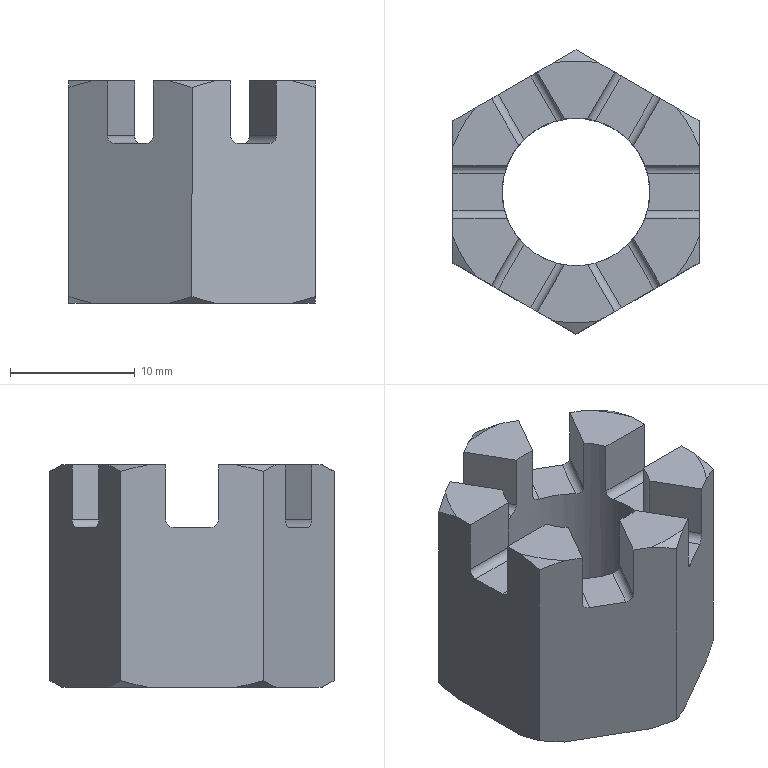Part | SolidWorks | features Cut 3, Chamfer 1, CirPattern 1, Extrusion 1 | 1 solid | 59 faces | box 19.728 x 22.78 x 17.8 mm | volume 3522 mm3 | plane 31 | cone 14 | cylinder 14 | commonest cylinder face diameters 1.25 x12 11.835 x2